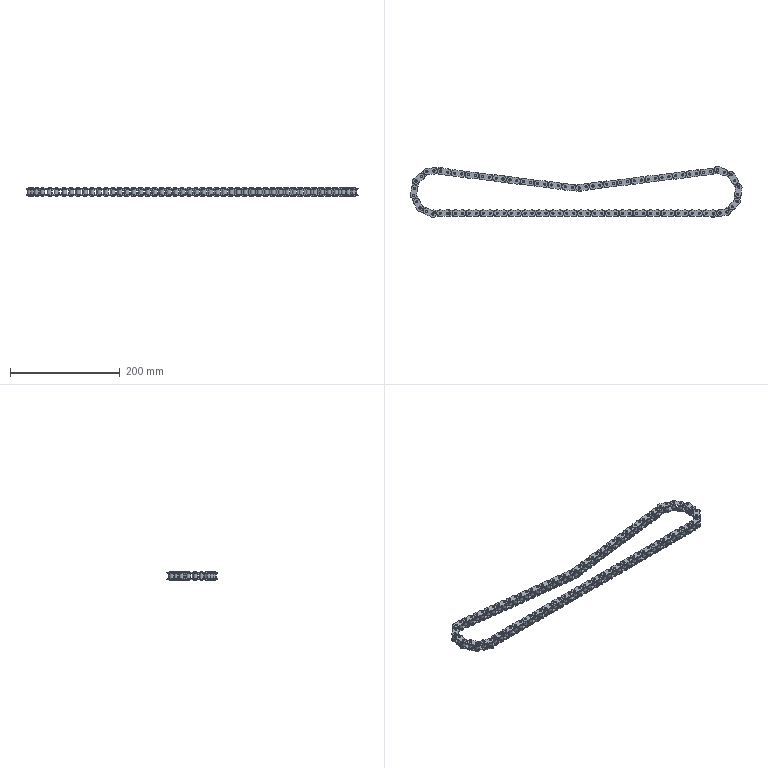Part | STEP file | Middle chain | 150 solids | 3000 faces | box 605.495 x 93.494 x 16.175 mm | volume 126775 mm3 | cylinder 2000 | plane 600 | cone 400 | commonest cylinder face diameters 3.98 x800 12.07 x600 55.348 x400 7.92 x200